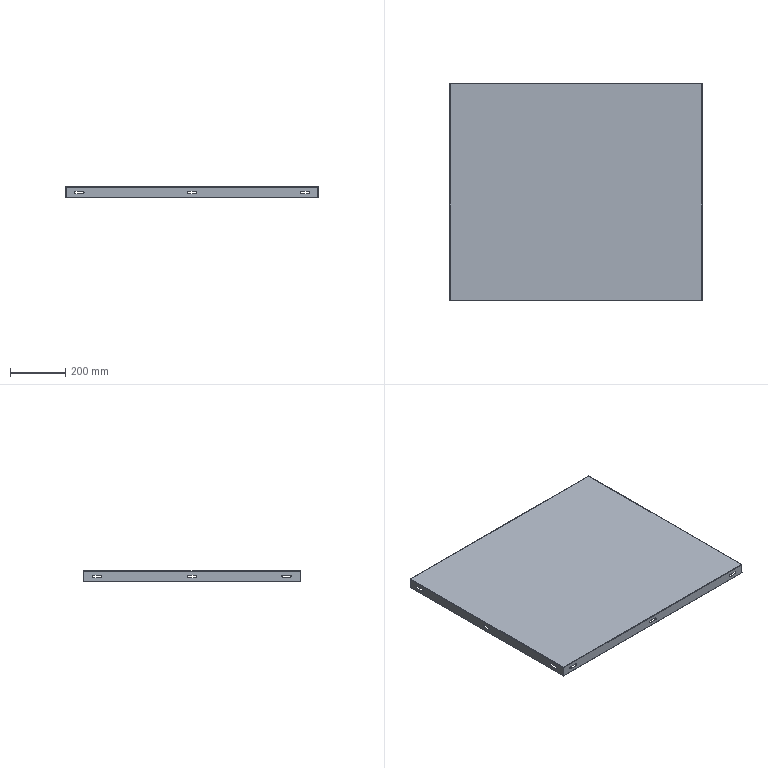Part | STEP file | Sheet-metal sealing plate_PN_0008 | 1 solid | 91 faces | box 919 x 789 x 38 mm | volume 1267247 mm3 | cylinder 36 | plane 35 | spline 20 | commonest cylinder face diameters 9 x24 0.2 x4 2 x4 3.2 x4